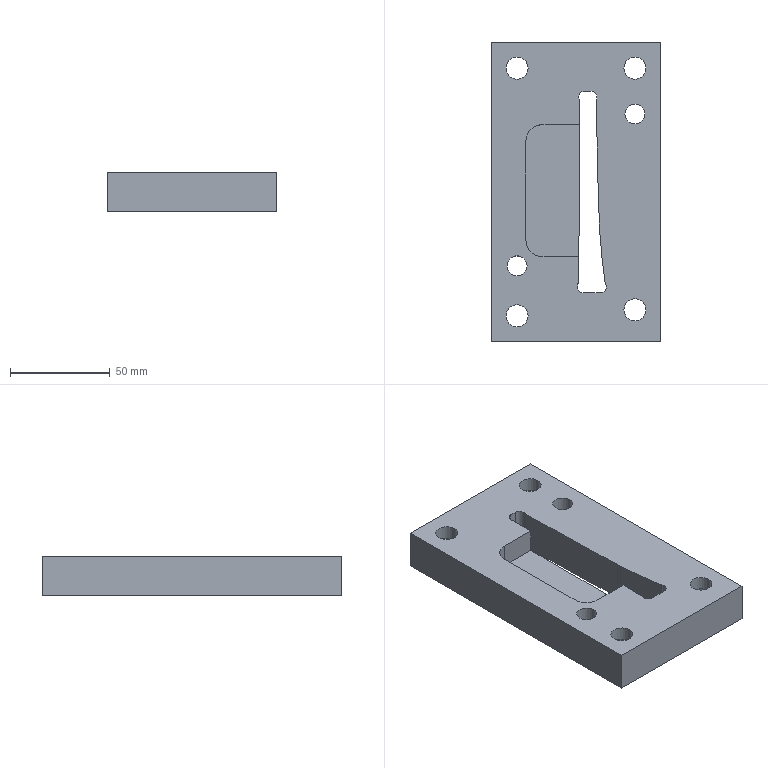Part | STEP file | 405_id2270_x_t | 1 solid | 48 faces | box 85 x 150 x 20 mm | volume 196124 mm3 | cylinder 22 | plane 21 | spline 5 | commonest cylinder face diameters 11 x6 4 x4 6 x4 17 x4 10 x2 16 x2